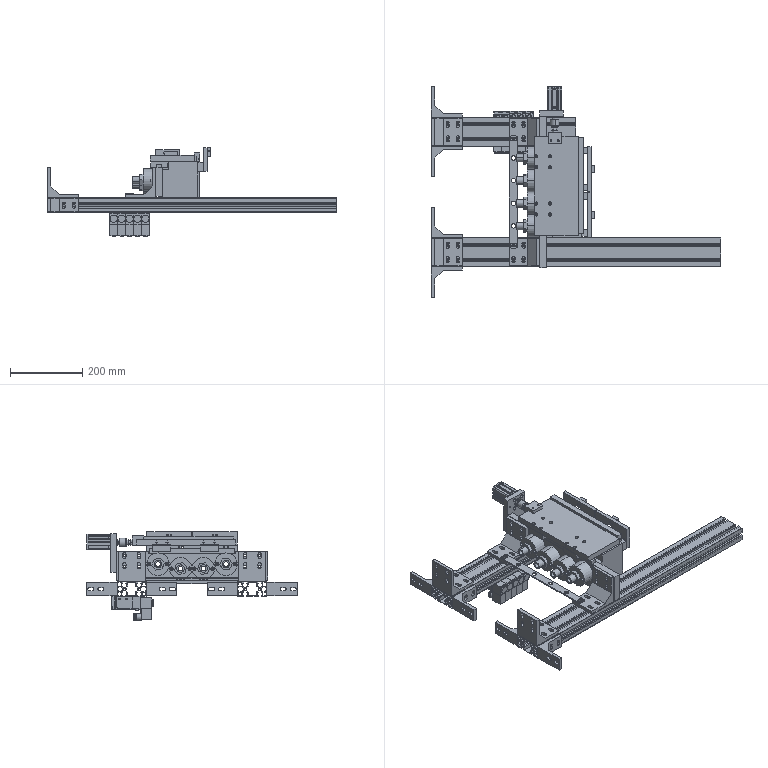Part | 46 solids | 2517 faces | box 800 x 584 x 246.4 mm | volume 5902281 mm3 | plane 1188 | cylinder 1054 | cone 241 | spline 28 | sphere 4 | torus 2 | commonest cylinder face diameters 9 x184 4.2 x96 2 x94 5.2 x52 11.445 x50 6 x39